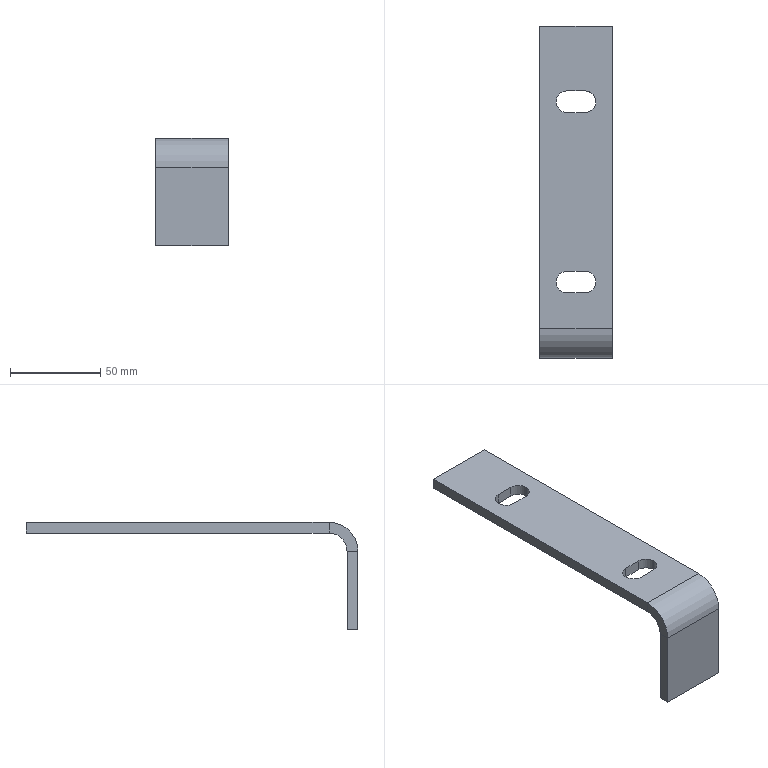Part | STEP file | 护栏连接Plate-250×125-1 | 1 solid | 24 faces | box 40 x 184 x 59.5 mm | volume 52864 mm3 | plane 16 | cylinder 8 | commonest cylinder face diameters 12 x6 20 x1 32 x1